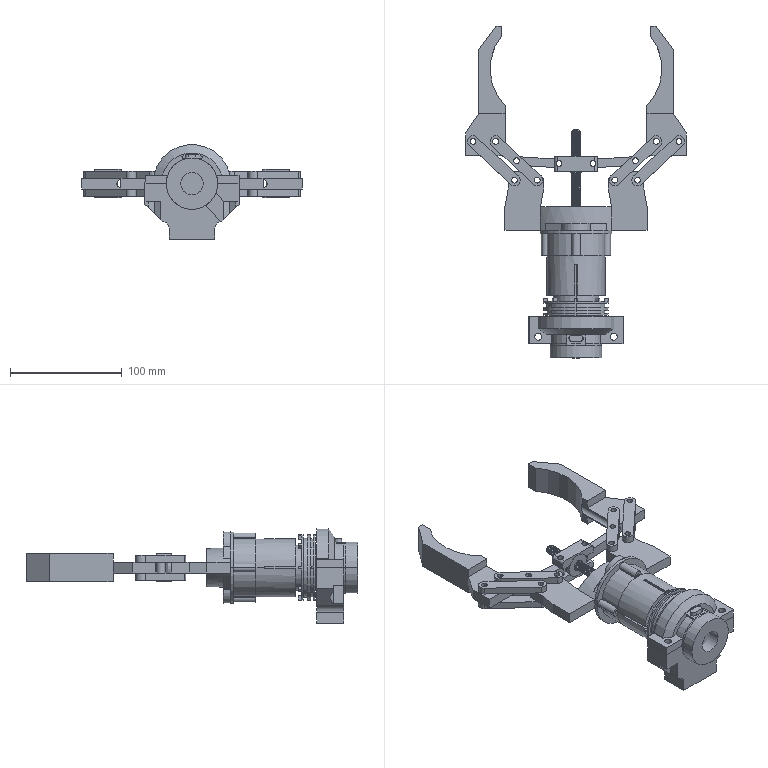Part | SolidWorks | features CompositeCurve 13, ReferencePattern 8, MirrorCompFeat 3, RefAxis 2 | 29 solids | 997 faces | box 197.047 x 296.861 x 84.62 mm | volume 451687 mm3 | plane 482 | cylinder 356 | spline 129 | cone 23 | torus 7 | commonest cylinder face diameters 6 x104 5.207 x72 2.8 x21 10.16 x16 52 x12 7.8 x9